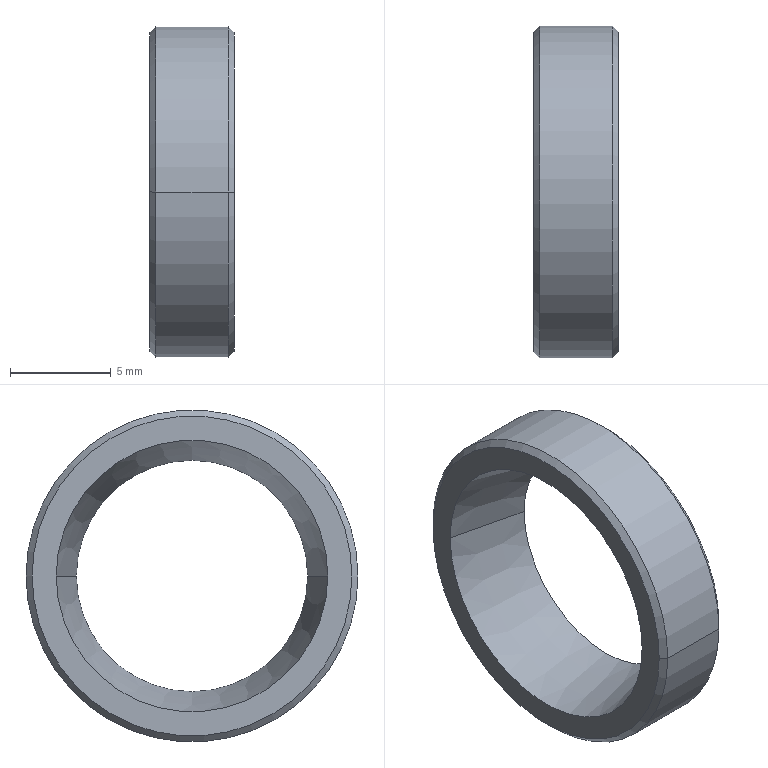Part | STEP file | part 10.stp.STEP-158.STEP | 1 solid | 10 faces | box 4.2 x 16.5 x 16.5 mm | volume 376.938 mm3 | cone 6 | cylinder 2 | plane 2 | commonest cylinder face diameters 16.5 x2
STEP:
#1=CARTESIAN_POINT('',(427.84,-7.95,0.));
#2=VERTEX_POINT('',#1);
#3=CARTESIAN_POINT('',(427.84,7.95,0.));
#4=VERTEX_POINT('',#3);
#5=CARTESIAN_POINT('',(427.84,0.,0.));
#6=DIRECTION('',(-1.,0.,0.));
#7=DIRECTION('',(0.,-1.,0.));
#8=AXIS2_PLACEMENT_3D('',#5,#6,#7);
#9=CIRCLE('',#8,7.95);
#10=EDGE_CURVE('',#2,#4,#9,.T.);
#11=ORIENTED_EDGE('',*,*,#10,.F.);
#12=CARTESIAN_POINT('',(428.14,-8.25,0.));
#13=VERTEX_POINT('',#12);
#14=CARTESIAN_POINT('',(428.14,-8.25,0.));
#15=DIRECTION('',(0.7071,-0.7071,0.));
#16=VECTOR('',#15,1000.);
#17=LINE('',#14,#16);
#18=EDGE_CURVE('',#2,#13,#17,.T.);
#19=ORIENTED_EDGE('',*,*,#18,.T.);
#20=CARTESIAN_POINT('',(428.14,8.25,0.));
#21=VERTEX_POINT('',#20);
#22=CARTESIAN_POINT('',(428.14,0.,0.));
#23=DIRECTION('',(1.,0.,0.));
#24=DIRECTION('',(0.,-1.,0.));
#25=AXIS2_PLACEMENT_3D('',#22,#23,#24);
#26=CIRCLE('',#25,8.25);
#27=EDGE_CURVE('',#21,#13,#26,.T.);
#28=ORIENTED_EDGE('',*,*,#27,.F.);
#29=CARTESIAN_POINT('',(428.14,8.25,0.));
#30=DIRECTION('',(0.7071,0.7071,0.));
#31=VECTOR('',#30,1000.);
#32=LINE('',#29,#31);
#33=EDGE_CURVE('',#4,#21,#32,.T.);
#34=ORIENTED_EDGE('',*,*,#33,.F.);
#35=EDGE_LOOP('',(#11,#19,#28,#34));
#36=FACE_OUTER_BOUND('',#35,.T.);
#37=CARTESIAN_POINT('',(428.14,0.,0.));
#38=DIRECTION('',(1.,0.,0.));
#39=DIRECTION('',(0.,1.,0.));
#40=AXIS2_PLACEMENT_3D('',#37,#38,#39);
#41=CONICAL_SURFACE('',#40,8.25,0.7854);
#42=ADVANCED_FACE('',(#36),#41,.T.);
#43=CARTESIAN_POINT('',(428.14,0.,0.));
#44=DIRECTION('',(1.,0.,0.));
#45=DIRECTION('',(0.,-1.,0.));
#46=AXIS2_PLACEMENT_3D('',#43,#44,#45);
#47=CIRCLE('',#46,8.25);
#48=EDGE_CURVE('',#13,#21,#47,.T.);
#49=ORIENTED_EDGE('',*,*,#48,.T.);
#50=CARTESIAN_POINT('',(431.74,8.25,0.));
#51=VERTEX_POINT('',#50);
#52=CARTESIAN_POINT('',(0.,8.25,0.));
#53=DIRECTION('',(1.,0.,0.));
#54=VECTOR('',#53,1000.);
#55=LINE('',#52,#54);
#56=EDGE_CURVE('',#21,#51,#55,.T.);
#57=ORIENTED_EDGE('',*,*,#56,.T.);
#58=CARTESIAN_POINT('',(431.74,-8.25,0.));
#59=VERTEX_POINT('',#58);
#60=CARTESIAN_POINT('',(431.74,0.,0.));
#61=DIRECTION('',(-1.,0.,0.));
#62=DIRECTION('',(0.,1.,0.));
#63=AXIS2_PLACEMENT_3D('',#60,#61,#62);
#64=CIRCLE('',#63,8.25);
#65=EDGE_CURVE('',#51,#59,#64,.T.);
#66=ORIENTED_EDGE('',*,*,#65,.T.);
#67=CARTESIAN_POINT('',(0.,-8.25,0.));
#68=DIRECTION('',(1.,0.,0.));
#69=VECTOR('',#68,1000.);
#70=LINE('',#67,#69);
#71=EDGE_CURVE('',#13,#59,#70,.T.);
#72=ORIENTED_EDGE('',*,*,#71,.F.);
#73=EDGE_LOOP('',(#49,#57,#66,#72));
#74=FACE_OUTER_BOUND('',#73,.T.);
#75=CARTESIAN_POINT('',(0.,0.,0.));
#76=DIRECTION('',(1.,0.,0.));
#77=DIRECTION('',(0.,-1.,0.));
#78=AXIS2_PLACEMENT_3D('',#75,#76,#77);
#79=CYLINDRICAL_SURFACE('',#78,8.25);
#80=ADVANCED_FACE('',(#74),#79,.T.);
#81=CARTESIAN_POINT('',(432.04,5.75,0.));
#82=VERTEX_POINT('',#81);
#83=CARTESIAN_POINT('',(432.04,-5.75,0.));
#84=VERTEX_POINT('',#83);
#85=CARTESIAN_POINT('',(432.04,0.,0.));
#86=DIRECTION('',(1.,0.,0.));
#87=DIRECTION('',(0.,-1.,0.));
#88=AXIS2_PLACEMENT_3D('',#85,#86,#87);
#89=CIRCLE('',#88,5.75);
#90=EDGE_CURVE('',#82,#84,#89,.T.);
#91=ORIENTED_EDGE('',*,*,#90,.T.);
#92=CARTESIAN_POINT('',(427.84,-6.75,0.));
#93=VERTEX_POINT('',#92);
#94=CARTESIAN_POINT('',(427.84,-6.75,0.));
#95=DIRECTION('',(-0.9728,-0.2316,0.));
#96=VECTOR('',#95,1000.);
#97=LINE('',#94,#96);
#98=EDGE_CURVE('',#84,#93,#97,.T.);
#99=ORIENTED_EDGE('',*,*,#98,.T.);
#100=CARTESIAN_POINT('',(427.84,6.75,0.));
#101=VERTEX_POINT('',#100);
#102=CARTESIAN_POINT('',(427.84,0.,0.));
#103=DIRECTION('',(1.,0.,0.));
#104=DIRECTION('',(0.,-1.,0.));
#105=AXIS2_PLACEMENT_3D('',#102,#103,#104);
#106=CIRCLE('',#105,6.75);
#107=EDGE_CURVE('',#101,#93,#106,.T.);
#108=ORIENTED_EDGE('',*,*,#107,.F.);
#109=CARTESIAN_POINT('',(427.84,6.75,0.));
#110=DIRECTION('',(-0.9728,0.2316,0.));
#111=VECTOR('',#110,1000.);
#112=LINE('',#109,#111);
#113=EDGE_CURVE('',#82,#101,#112,.T.);
#114=ORIENTED_EDGE('',*,*,#113,.F.);
#115=EDGE_LOOP('',(#91,#99,#108,#114));
#116=FACE_OUTER_BOUND('',#115,.T.);
#117=CARTESIAN_POINT('',(427.84,0.,0.));
#118=DIRECTION('',(-1.,0.,0.));
#119=DIRECTION('',(0.,1.,0.));
#120=AXIS2_PLACEMENT_3D('',#117,#118,#119);
#121=CONICAL_SURFACE('',#120,6.75,0.2337);
#122=ADVANCED_FACE('',(#116),#121,.F.);
#123=CARTESIAN_POINT('',(432.04,7.95,0.));
#124=VERTEX_POINT('',#123);
#125=CARTESIAN_POINT('',(432.04,-7.95,0.));
#126=VERTEX_POINT('',#125);
#127=CARTESIAN_POINT('',(432.04,0.,0.));
#128=DIRECTION('',(1.,0.,0.));
#129=DIRECTION('',(0.,1.,0.));
#130=AXIS2_PLACEMENT_3D('',#127,#128,#129);
#131=CIRCLE('',#130,7.95);
#132=EDGE_CURVE('',#124,#126,#131,.T.);
#133=ORIENTED_EDGE('',*,*,#132,.F.);
#134=CARTESIAN_POINT('',(432.04,7.95,0.));
#135=DIRECTION('',(-0.7071,0.7071,0.));
#136=VECTOR('',#135,1000.);
#137=LINE('',#134,#136);
#138=EDGE_CURVE('',#124,#51,#137,.T.);
#139=ORIENTED_EDGE('',*,*,#138,.T.);
#140=CARTESIAN_POINT('',(431.74,0.,0.));
#141=DIRECTION('',(-1.,0.,0.));
#142=DIRECTION('',(0.,1.,0.));
#143=AXIS2_PLACEMENT_3D('',#140,#141,#142);
#144=CIRCLE('',#143,8.25);
#145=EDGE_CURVE('',#59,#51,#144,.T.);
#146=ORIENTED_EDGE('',*,*,#145,.F.);
#147=CARTESIAN_POINT('',(432.04,-7.95,0.));
#148=DIRECTION('',(-0.7071,-0.7071,0.));
#149=VECTOR('',#148,1000.);
#150=LINE('',#147,#149);
#151=EDGE_CURVE('',#126,#59,#150,.T.);
#152=ORIENTED_EDGE('',*,*,#151,.F.);
#153=EDGE_LOOP('',(#133,#139,#146,#152));
#154=FACE_OUTER_BOUND('',#153,.T.);
#155=CARTESIAN_POINT('',(432.04,0.,0.));
#156=DIRECTION('',(-1.,0.,0.));
#157=DIRECTION('',(0.,-1.,0.));
#158=AXIS2_PLACEMENT_3D('',#155,#156,#157);
#159=CONICAL_SURFACE('',#158,7.95,0.7854);
#160=ADVANCED_FACE('',(#154),#159,.T.);
#161=ORIENTED_EDGE('',*,*,#138,.F.);
#162=CARTESIAN_POINT('',(432.04,0.,0.));
#163=DIRECTION('',(1.,0.,0.));
#164=DIRECTION('',(0.,1.,0.));
#165=AXIS2_PLACEMENT_3D('',#162,#163,#164);
#166=CIRCLE('',#165,7.95);
#167=EDGE_CURVE('',#126,#124,#166,.T.);
#168=ORIENTED_EDGE('',*,*,#167,.F.);
#169=ORIENTED_EDGE('',*,*,#151,.T.);
#170=ORIENTED_EDGE('',*,*,#65,.F.);
#171=EDGE_LOOP('',(#161,#168,#169,#170));
#172=FACE_OUTER_BOUND('',#171,.T.);
#173=CARTESIAN_POINT('',(432.04,0.,0.));
#174=DIRECTION('',(-1.,0.,0.));
#175=DIRECTION('',(0.,-1.,0.));
#176=AXIS2_PLACEMENT_3D('',#173,#174,#175);
#177=CONICAL_SURFACE('',#176,7.95,0.7854);
#178=ADVANCED_FACE('',(#172),#177,.T.);
#179=ORIENTED_EDGE('',*,*,#98,.F.);
#180=CARTESIAN_POINT('',(432.04,0.,0.));
#181=DIRECTION('',(1.,0.,0.));
#182=DIRECTION('',(0.,-1.,0.));
#183=AXIS2_PLACEMENT_3D('',#180,#181,#182);
#184=CIRCLE('',#183,5.75);
#185=EDGE_CURVE('',#84,#82,#184,.T.);
#186=ORIENTED_EDGE('',*,*,#185,.T.);
#187=ORIENTED_EDGE('',*,*,#113,.T.);
#188=CARTESIAN_POINT('',(427.84,0.,0.));
#189=DIRECTION('',(1.,0.,0.));
#190=DIRECTION('',(0.,-1.,0.));
#191=AXIS2_PLACEMENT_3D('',#188,#189,#190);
#192=CIRCLE('',#191,6.75);
#193=EDGE_CURVE('',#93,#101,#192,.T.);
#194=ORIENTED_EDGE('',*,*,#193,.F.);
#195=EDGE_LOOP('',(#179,#186,#187,#194));
#196=FACE_OUTER_BOUND('',#195,.T.);
#197=CARTESIAN_POINT('',(427.84,0.,0.));
#198=DIRECTION('',(-1.,0.,0.));
#199=DIRECTION('',(0.,1.,0.));
#200=AXIS2_PLACEMENT_3D('',#197,#198,#199);
#201=CONICAL_SURFACE('',#200,6.75,0.2337);
#202=ADVANCED_FACE('',(#196),#201,.F.);
#203=ORIENTED_EDGE('',*,*,#107,.T.);
#204=ORIENTED_EDGE('',*,*,#193,.T.);
#205=EDGE_LOOP('',(#203,#204));
#206=FACE_BOUND('',#205,.T.);
#207=CARTESIAN_POINT('',(427.84,0.,0.));
#208=DIRECTION('',(-1.,0.,0.));
#209=DIRECTION('',(0.,-1.,0.));
#210=AXIS2_PLACEMENT_3D('',#207,#208,#209);
#211=CIRCLE('',#210,7.95);
#212=EDGE_CURVE('',#4,#2,#211,.T.);
#213=ORIENTED_EDGE('',*,*,#212,.T.);
#214=ORIENTED_EDGE('',*,*,#10,.T.);
#215=EDGE_LOOP('',(#213,#214));
#216=FACE_OUTER_BOUND('',#215,.T.);
#217=CARTESIAN_POINT('',(427.84,8.25,0.));
#218=DIRECTION('',(-1.,0.,0.));
#219=DIRECTION('',(0.,1.,0.));
#220=AXIS2_PLACEMENT_3D('',#217,#218,#219);
#221=PLANE('',#220);
#222=ADVANCED_FACE('',(#206,#216),#221,.T.);
#223=ORIENTED_EDGE('',*,*,#90,.F.);
#224=ORIENTED_EDGE('',*,*,#185,.F.);
#225=EDGE_LOOP('',(#223,#224));
#226=FACE_BOUND('',#225,.T.);
#227=ORIENTED_EDGE('',*,*,#167,.T.);
#228=ORIENTED_EDGE('',*,*,#132,.T.);
#229=EDGE_LOOP('',(#227,#228));
#230=FACE_OUTER_BOUND('',#229,.T.);
#231=CARTESIAN_POINT('',(432.04,5.75,0.));
#232=DIRECTION('',(1.,0.,0.));
#233=DIRECTION('',(0.,1.,0.));
#234=AXIS2_PLACEMENT_3D('',#231,#232,#233);
#235=PLANE('',#234);
#236=ADVANCED_FACE('',(#226,#230),#235,.T.);
#237=ORIENTED_EDGE('',*,*,#56,.F.);
#238=ORIENTED_EDGE('',*,*,#27,.T.);
#239=ORIENTED_EDGE('',*,*,#71,.T.);
#240=ORIENTED_EDGE('',*,*,#145,.T.);
#241=EDGE_LOOP('',(#237,#238,#239,#240));
#242=FACE_OUTER_BOUND('',#241,.T.);
#243=CARTESIAN_POINT('',(0.,0.,0.));
#244=DIRECTION('',(1.,0.,0.));
#245=DIRECTION('',(0.,-1.,0.));
#246=AXIS2_PLACEMENT_3D('',#243,#244,#245);
#247=CYLINDRICAL_SURFACE('',#246,8.25);
#248=ADVANCED_FACE('',(#242),#247,.T.);
#249=ORIENTED_EDGE('',*,*,#18,.F.);
#250=ORIENTED_EDGE('',*,*,#212,.F.);
#251=ORIENTED_EDGE('',*,*,#33,.T.);
#252=ORIENTED_EDGE('',*,*,#48,.F.);
#253=EDGE_LOOP('',(#249,#250,#251,#252));
#254=FACE_OUTER_BOUND('',#253,.T.);
#255=CARTESIAN_POINT('',(428.14,0.,0.));
#256=DIRECTION('',(1.,0.,0.));
#257=DIRECTION('',(0.,1.,0.));
#258=AXIS2_PLACEMENT_3D('',#255,#256,#257);
#259=CONICAL_SURFACE('',#258,8.25,0.7854);
#260=ADVANCED_FACE('',(#254),#259,.T.);
#261=CLOSED_SHELL('',(#42,#80,#122,#160,#178,#202,#222,#236,#248,#260));
#262=MANIFOLD_SOLID_BREP('',#261);
#263=CARTESIAN_POINT('',(0.,0.,0.));
#264=DIRECTION('',(0.,0.,1.));
#265=DIRECTION('',(1.,0.,0.));
#266=AXIS2_PLACEMENT_3D('',#263,#264,#265);
#267=(LENGTH_UNIT()NAMED_UNIT(*)SI_UNIT(.MILLI.,.METRE.));
#268=UNCERTAINTY_MEASURE_WITH_UNIT(LENGTH_MEASURE(0.00001),#267,'','');
#269=(NAMED_UNIT(*)PLANE_ANGLE_UNIT()SI_UNIT($,.RADIAN.));
#270=(NAMED_UNIT(*)SI_UNIT($,.STERADIAN.)SOLID_ANGLE_UNIT());
#271=(GEOMETRIC_REPRESENTATION_CONTEXT(3)GLOBAL_UNCERTAINTY_ASSIGNED_CONTEXT((#268))GLOBAL_UNIT_ASSIGNED_CONTEXT((#267,#269,#270))REPRESENTATION_CONTEXT('',''));
#272=ADVANCED_BREP_SHAPE_REPRESENTATION('',(#262,#266),#271);